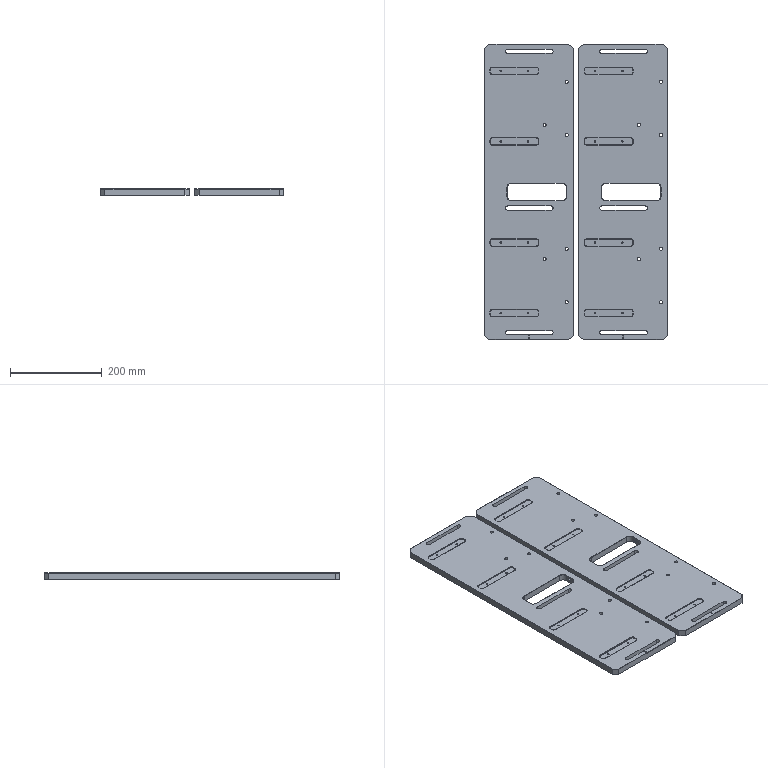NC program | NX | posted by the shop | part box 401 x 645 x 14 mm
Lines 4204 to 5636 of 5636:
N5 T02 M06
(D6 chamfer mill  D=6. R=0. H=02 ce=0.00 di=0.00)
G00 G90 G54 X-240.5 Y-185.9 M03 S3000
G43 H02 Z34.
M08
G98 G81 X-240.5 Y-185.9 Z11. R15. F200.
X-146.5 Y-137.4
X-124.5 Y-185.9
Y20.1
X-146.5 Y68.6
X-240.5 Y20.1
X124.5
X146.5 Y68.6
X240.5 Y20.1
X146.5 Y-137.4
X124.5 Y-185.9
X240.5
G80
G00 Z34.
G00 G90 X-310.789 Y102.451 M03 S6000
Z34.
Z16.934
G01 Z12.501 F1200.
X-310.731 Y102.283
X-310.7 Y102.
Y54.5
G03 X-307.5 Y51.3 I3.2 J0.0
X-304.3 Y54.5 I0.0 J3.2
G01 Y149.5
G03 X-307.5 Y152.7 I-3.2 J0.0
X-310.7 Y149.5 I0.0 J-3.2
G01 Y104.
X-310.731 Y103.717
X-310.789 Y103.549
Z16.934
G00 Z34.
X-37.372 Y102.25
Z16.099
G01 Z12.501
G03 X-37.672 Y102.33 I-.3 J-.52
X-38.192 Y102.03 I0.0 J-.6
G01 X-38.2 Y102.
Y54.5
G03 X-35. Y51.3 I3.2 J0.0
X-31.8 Y54.5 I0.0 J3.2
G01 Y149.5
G03 X-35. Y152.7 I-3.2 J0.0
X-38.2 Y149.5 I0.0 J-3.2
G01 Y102.
X-38.192 Y101.97
G03 X-37.672 Y101.67 I.52 J.3
X-37.372 Y101.75 I0.0 J.6
G01 Z16.099
G00 Z34.
X305.128 Y102.25
Z16.099
G01 Z12.501
G03 X304.828 Y102.33 I-.3 J-.52
X304.308 Y102.03 I0.0 J-.6
G01 X304.3 Y102.
Y54.5
G03 X307.5 Y51.3 I3.2 J0.0
X310.7 Y54.5 I0.0 J3.2
G01 Y149.5
G03 X307.5 Y152.7 I-3.2 J0.0
X304.3 Y149.5 I0.0 J-3.2
G01 Y102.
X304.308 Y101.97
G03 X304.828 Y101.67 I.52 J.3
X305.128 Y101.75 I0.0 J.6
G01 Z16.099
G00 Z34.
X-310.789 Y-103.549
Z16.934
G01 Z12.501
X-310.731 Y-103.717
X-310.7 Y-104.
Y-151.5
G03 X-307.5 Y-154.7 I3.2 J0.0
X-304.3 Y-151.5 I0.0 J3.2
G01 Y-56.5
G03 X-307.5 Y-53.3 I-3.2 J0.0
X-310.7 Y-56.5 I0.0 J-3.2
G01 Y-102.
X-310.731 Y-102.283
X-310.789 Y-102.451
Z16.934
G00 Z34.
X-37.372 Y-103.75
Z16.099
G01 Z12.501
G03 X-37.672 Y-103.67 I-.3 J-.52
X-38.192 Y-103.97 I0.0 J-.6
G01 X-38.2 Y-104.
Y-151.5
G03 X-35. Y-154.7 I3.2 J0.0
X-31.8 Y-151.5 I0.0 J3.2
G01 Y-56.5
G03 X-35. Y-53.3 I-3.2 J0.0
X-38.2 Y-56.5 I0.0 J-3.2
G01 Y-104.
X-38.192 Y-104.03
G03 X-37.672 Y-104.33 I.52 J.3
X-37.372 Y-104.25 I0.0 J.6
G01 Z16.099
G00 Z34.
X305.128 Y-103.75
Z16.099
G01 Z12.501
G03 X304.828 Y-103.67 I-.3 J-.52
X304.308 Y-103.97 I0.0 J-.6
G01 X304.3 Y-104.
Y-151.5
G03 X307.5 Y-154.7 I3.2 J0.0
X310.7 Y-151.5 I0.0 J3.2
G01 Y-56.5
G03 X307.5 Y-53.3 I-3.2 J0.0
X304.3 Y-56.5 I0.0 J-3.2
G01 Y-104.
X304.308 Y-104.03
G03 X304.828 Y-104.33 I.52 J.3
X305.128 Y-104.25 I0.0 J.6
G01 Z16.099
G00 Z34.
G00 G90 X-264.5 Y-101.5 M03 S5000
Z34.
G98 G81 X-264.5 Y-101.5 Z9.85 R15. F150.
Y-41.5
Y104.5
Y164.5
X-110.5
Y104.5
Y-41.5
Y-101.5
X110.5
Y-41.5
Y104.5
Y164.5
X264.5
Y104.5
Y-41.5
Y-101.5
G80
G00 Z34.
G00 G90 X-242. Y-186.895 M03 S6000
Z34.
Z12.9
G01 Z12.4 F600.
Y-187.2
G03 X-240.5 Y-188.7 I1.5 J0.0
X-237.7 Y-185.9 I0.0 J2.8
X-240.5 Y-183.1 I-2.8 J0.0
X-243.3 Y-185.9 I0.0 J-2.8
X-240.5 Y-188.7 I2.8 J0.0
X-239. Y-187.2 I0.0 J1.5
G01 Y-186.895
Z12.9
G00 Z34.
X-126.
Z12.9
G01 Z12.4
Y-187.2
G03 X-124.5 Y-188.7 I1.5 J0.0
X-121.7 Y-185.9 I0.0 J2.8
X-124.5 Y-183.1 I-2.8 J0.0
X-127.3 Y-185.9 I0.0 J-2.8
X-124.5 Y-188.7 I2.8 J0.0
X-123. Y-187.2 I0.0 J1.5
G01 Y-186.895
Z12.9
G00 Z34.
X-148. Y-138.395
Z12.9
G01 Z12.4
Y-138.7
G03 X-146.5 Y-140.2 I1.5 J0.0
X-143.7 Y-137.4 I0.0 J2.8
X-146.5 Y-134.6 I-2.8 J0.0
X-149.3 Y-137.4 I0.0 J-2.8
X-146.5 Y-140.2 I2.8 J0.0
X-145. Y-138.7 I0.0 J1.5
G01 Y-138.395
Z12.9
G00 Z34.
X-242. Y19.105
Z12.9
G01 Z12.4
Y18.8
G03 X-240.5 Y17.3 I1.5 J0.0
X-237.7 Y20.1 I0.0 J2.8
X-240.5 Y22.9 I-2.8 J0.0
X-243.3 Y20.1 I0.0 J-2.8
X-240.5 Y17.3 I2.8 J0.0
X-239. Y18.8 I0.0 J1.5
G01 Y19.105
Z12.9
G00 Z34.
X-148. Y67.605
Z12.9
G01 Z12.4
Y67.3
G03 X-146.5 Y65.8 I1.5 J0.0
X-143.7 Y68.6 I0.0 J2.8
X-146.5 Y71.4 I-2.8 J0.0
X-149.3 Y68.6 I0.0 J-2.8
X-146.5 Y65.8 I2.8 J0.0
X-145. Y67.3 I0.0 J1.5
G01 Y67.605
Z12.9
G00 Z34.
X-126. Y19.105
Z12.9
G01 Z12.4
Y18.8
G03 X-124.5 Y17.3 I1.5 J0.0
X-121.7 Y20.1 I0.0 J2.8
X-124.5 Y22.9 I-2.8 J0.0
X-127.3 Y20.1 I0.0 J-2.8
X-124.5 Y17.3 I2.8 J0.0
X-123. Y18.8 I0.0 J1.5
G01 Y19.105
Z12.9
G00 Z34.
X123.
Z12.9
G01 Z12.4
Y18.8
G03 X124.5 Y17.3 I1.5 J0.0
X127.3 Y20.1 I0.0 J2.8
X124.5 Y22.9 I-2.8 J0.0
X121.7 Y20.1 I0.0 J-2.8
X124.5 Y17.3 I2.8 J0.0
X126. Y18.8 I0.0 J1.5
G01 Y19.105
Z12.9
G00 Z34.
X145. Y67.605
Z12.9
G01 Z12.4
Y67.3
G03 X146.5 Y65.8 I1.5 J0.0
X149.3 Y68.6 I0.0 J2.8
X146.5 Y71.4 I-2.8 J0.0
X143.7 Y68.6 I0.0 J-2.8
X146.5 Y65.8 I2.8 J0.0
X148. Y67.3 I0.0 J1.5
G01 Y67.605
Z12.9
G00 Z34.
X239. Y19.105
Z12.9
G01 Z12.4
Y18.8
G03 X240.5 Y17.3 I1.5 J0.0
X243.3 Y20.1 I0.0 J2.8
X240.5 Y22.9 I-2.8 J0.0
X237.7 Y20.1 I0.0 J-2.8
X240.5 Y17.3 I2.8 J0.0
X242. Y18.8 I0.0 J1.5
G01 Y19.105
Z12.9
G00 Z34.
X145. Y-138.395
Z12.9
G01 Z12.4
Y-138.7
G03 X146.5 Y-140.2 I1.5 J0.0
X149.3 Y-137.4 I0.0 J2.8
X146.5 Y-134.6 I-2.8 J0.0
X143.7 Y-137.4 I0.0 J-2.8
X146.5 Y-140.2 I2.8 J0.0
X148. Y-138.7 I0.0 J1.5
G01 Y-138.395
Z12.9
G00 Z34.
X123. Y-186.895
Z12.9
G01 Z12.4
Y-187.2
G03 X124.5 Y-188.7 I1.5 J0.0
X127.3 Y-185.9 I0.0 J2.8
X124.5 Y-183.1 I-2.8 J0.0
X121.7 Y-185.9 I0.0 J-2.8
X124.5 Y-188.7 I2.8 J0.0
X126. Y-187.2 I0.0 J1.5
G01 Y-186.895
Z12.9
G00 Z34.
X239.
Z12.9
G01 Z12.4
Y-187.2
G03 X240.5 Y-188.7 I1.5 J0.0
X243.3 Y-185.9 I0.0 J2.8
X240.5 Y-183.1 I-2.8 J0.0
X237.7 Y-185.9 I0.0 J-2.8
X240.5 Y-188.7 I2.8 J0.0
X242. Y-187.2 I0.0 J1.5
G01 Y-186.895
Z12.9
G00 Z34.
G00 G90 X-313.126 Y4.753 M03 S6500
Z34.
Z16.501
G01 Z12.501 F1500.
X-313.354 Y4.939
X-323.061 Y14.646
X-323.247 Y14.874
Z16.501
G00 X-323.471 Y15.414
G01 Z12.501
X-323.5 Y15.707
Y102.
X-323.475 Y102.272
Z16.501
G00 Y103.728
G01 Z12.501
X-323.5 Y104.
Y190.293
X-323.471 Y190.586
Z16.501
G00 X-323.247 Y191.126
G01 Z12.501
X-323.061 Y191.354
X-313.354 Y201.061
X-313.126 Y201.247
Z16.501
G00 X-312.586 Y201.471
G01 Z12.501
X-312.293 Y201.5
X312.293
X312.586 Y201.471
Z16.501
G00 X313.126 Y201.247
G01 Z12.501
X313.354 Y201.061
X323.06 Y191.354
X323.247 Y191.126
Z16.501
G00 X323.471 Y190.586
G01 Z12.501
X323.5 Y190.293
Y15.707
X323.471 Y15.414
Z16.501
G00 X323.247 Y14.874
G01 Z12.501
X323.061 Y14.646
X313.354 Y4.939
X313.126 Y4.753
Z16.501
G00 X312.586 Y4.529
G01 Z12.501
X312.293 Y4.5
X0.0
X-312.293
X-312.586 Y4.529
Z16.501
G00 Z24.
X-304.727 Y101.614
Z13.672
G01 Z12.501
G03 X-304.527 Y101.9 I-1.532 J1.286
G01 X-304.497 Y101.946
X-304.5 Y102.
Y149.5
G03 X-307.5 Y152.5 I-3. J0.0
X-310.5 Y149.5 I0.0 J-3.
G01 Y104.
X-310.525 Y103.728
X-310.599 Y103.465
X-310.719 Y103.219
X-310.882 Y103.
X-310.719 Y102.781
X-310.599 Y102.535
X-310.525 Y102.272
X-310.5 Y102.
Y54.5
G03 X-307.5 Y51.5 I3. J0.0
X-304.5 Y54.5 I0.0 J3.
G01 Y102.
X-304.497 Y102.054
X-304.527 Y102.1
G03 X-304.727 Y102.386 I-1.732 J-1.
G01 Z13.672
G00 Z24.
X-270.873 Y134.886
Z13.672
G01 Z12.501
G03 X-271.073 Y134.6 I1.532 J-1.286
G01 X-271.103 Y134.554
X-271.1 Y134.5
Y86.5
G03 X-267.1 Y82.5 I4. J0.0
G01 X-261.9
G03 X-257.9 Y86.5 I0.0 J4.
G01 Y182.5
G03 X-261.9 Y186.5 I-4. J0.0
G01 X-267.1
G03 X-271.1 Y182.5 I0.0 J-4.
G01 Y134.5
X-271.103 Y134.446
X-271.073 Y134.4
G03 X-270.873 Y134.114 I1.732 J1.
G01 Z13.672
G00 Z24.
X-240.904 Y18.392
Z13.759
G01 Z12.501
G03 X-240.602 Y18.218 I1.147 J1.638
G01 X-240.554 Y18.192
X-240.5 Y18.2
G03 X-238.6 Y20.1 I0.0 J1.9
X-240.5 Y22. I-1.9 J0.0
X-242.4 Y20.1 I0.0 J-1.9
X-240.83 Y18.229 I1.9 J0.0
G01 X-240.5 Y18.2
X-240.446 Y18.192
X-240.398 Y18.218
G03 X-240.096 Y18.392 I-.845 J1.813
G01 Z13.759
G00 Z24.
X-124.904
Z13.759
G01 Z12.501
G03 X-124.602 Y18.218 I1.147 J1.638
G01 X-124.554 Y18.192
X-124.5 Y18.2
G03 X-122.6 Y20.1 I0.0 J1.9
X-124.5 Y22. I-1.9 J0.0
X-126.4 Y20.1 I0.0 J-1.9
X-124.83 Y18.229 I1.9 J0.0
G01 X-124.5 Y18.2
X-124.446 Y18.192
X-124.398 Y18.218
G03 X-124.096 Y18.392 I-.845 J1.813
G01 Z13.759
G00 Z24.
X-146.904 Y66.892
Z13.759
G01 Z12.501
G03 X-146.602 Y66.718 I1.147 J1.638
G01 X-146.554 Y66.692
X-146.5 Y66.7
G03 X-144.6 Y68.6 I0.0 J1.9
X-146.5 Y70.5 I-1.9 J0.0
X-148.4 Y68.6 I0.0 J-1.9
X-146.83 Y66.729 I1.9 J0.0
G01 X-146.5 Y66.7
X-146.446 Y66.692
X-146.398 Y66.718
G03 X-146.096 Y66.892 I-.845 J1.813
G01 Z13.759
G00 Z24.
X-116.873 Y134.886
Z13.672
G01 Z12.501
G03 X-117.073 Y134.6 I1.532 J-1.286
G01 X-117.103 Y134.554
X-117.1 Y134.5
Y86.5
G03 X-113.1 Y82.5 I4. J0.0
G01 X-107.9
G03 X-103.9 Y86.5 I0.0 J4.
G01 Y182.5
G03 X-107.9 Y186.5 I-4. J0.0
G01 X-113.1
G03 X-117.1 Y182.5 I0.0 J-4.
G01 Y134.5
X-117.103 Y134.446
X-117.073 Y134.4
G03 X-116.873 Y134.114 I1.732 J1.
G01 Z13.672
G00 Z24.
X-37.773 Y102.386
Z13.672
G01 Z12.501
G03 X-37.973 Y102.1 I1.532 J-1.286
G01 X-38.003 Y102.054
X-38. Y102.
Y54.5
G03 X-35. Y51.5 I3. J0.0
X-32. Y54.5 I0.0 J3.
G01 Y149.5
G03 X-35. Y152.5 I-3. J0.0
X-38. Y149.5 I0.0 J-3.
G01 Y102.
X-38.003 Y101.946
X-37.973 Y101.9
G03 X-37.773 Y101.614 I1.732 J1.
G01 Z13.672
G00 Z24.
X-17.773 Y85.886
Z13.672
G01 Z12.501
G03 X-17.973 Y85.6 I1.532 J-1.286
G01 X-18.003 Y85.554
X-18. Y85.5
Y30.5
G03 X-9. Y21.5 I9. J0.0
G01 X9.
G03 X18. Y30.5 I0.0 J9.
G01 Y140.5
G03 X9. Y149.5 I-9. J0.0
G01 X-9.
G03 X-18. Y140.5 I0.0 J-9.
G01 Y85.5
X-18.003 Y85.446
X-17.973 Y85.4
G03 X-17.773 Y85.114 I1.732 J1.
G01 Z13.672
G00 Z24.
X104.127 Y134.886
Z13.672
G01 Z12.501
G03 X103.927 Y134.6 I1.532 J-1.286
G01 X103.897 Y134.554
X103.9 Y134.5
Y86.5
G03 X107.9 Y82.5 I4. J0.0
G01 X113.1
G03 X117.1 Y86.5 I0.0 J4.
G01 Y182.5
G03 X113.1 Y186.5 I-4. J0.0
G01 X107.9
G03 X103.9 Y182.5 I0.0 J-4.
G01 Y134.5
X103.897 Y134.446
X103.927 Y134.4
G03 X104.127 Y134.114 I1.732 J1.
G01 Z13.672
G00 Z24.
X146.096 Y66.892
Z13.759
G01 Z12.501
G03 X146.398 Y66.718 I1.147 J1.638
G01 X146.446 Y66.692
X146.5 Y66.7
G03 X148.4 Y68.6 I0.0 J1.9
X146.5 Y70.5 I-1.9 J0.0
X144.6 Y68.6 I0.0 J-1.9
X146.17 Y66.729 I1.9 J0.0
G01 X146.5 Y66.7
X146.554 Y66.692
X146.602 Y66.718
G03 X146.904 Y66.892 I-.845 J1.813
G01 Z13.759
G00 Z24.
X124.096 Y18.392
Z13.759
G01 Z12.501
G03 X124.398 Y18.218 I1.147 J1.638
G01 X124.446 Y18.192
X124.5 Y18.2
G03 X126.4 Y20.1 I0.0 J1.9
X124.5 Y22. I-1.9 J0.0
X122.6 Y20.1 I0.0 J-1.9
X124.17 Y18.229 I1.9 J0.0
G01 X124.5 Y18.2
X124.554 Y18.192
X124.602 Y18.218
G03 X124.904 Y18.392 I-.845 J1.813
G01 Z13.759
G00 Z24.
X240.096
Z13.759
G01 Z12.501
G03 X240.398 Y18.218 I1.147 J1.638
G01 X240.446 Y18.192
X240.5 Y18.2
G03 X242.4 Y20.1 I0.0 J1.9
X240.5 Y22. I-1.9 J0.0
X238.6 Y20.1 I0.0 J-1.9
X240.17 Y18.229 I1.9 J0.0
G01 X240.5 Y18.2
X240.554 Y18.192
X240.602 Y18.218
G03 X240.904 Y18.392 I-.845 J1.813
G01 Z13.759
G00 Z24.
X304.727 Y102.386
Z13.672
G01 Z12.501
G03 X304.527 Y102.1 I1.532 J-1.286
G01 X304.497 Y102.054
X304.5 Y102.
Y54.5
G03 X307.5 Y51.5 I3. J0.0
X310.5 Y54.5 I0.0 J3.
G01 Y149.5
G03 X307.5 Y152.5 I-3. J0.0
X304.5 Y149.5 I0.0 J-3.
G01 Y102.
X304.497 Y101.946
X304.527 Y101.9
G03 X304.727 Y101.614 I1.732 J1.
G01 Z13.672
G00 Z24.
X270.873 Y134.114
Z13.672
G01 Z12.501
G03 X271.073 Y134.4 I-1.532 J1.286
G01 X271.103 Y134.446
X271.1 Y134.5
Y182.5
G03 X267.1 Y186.5 I-4. J0.0
G01 X261.9
G03 X257.9 Y182.5 I0.0 J-4.
G01 Y86.5
G03 X261.9 Y82.5 I4. J0.0
G01 X267.1
G03 X271.1 Y86.5 I0.0 J4.
G01 Y134.5
X271.103 Y134.554
X271.073 Y134.6
G03 X270.873 Y134.886 I-1.732 J-1.
G01 Z13.672
G00 Z24.
X313.126 Y-4.753
Z16.501
G01 Z12.501
X313.354 Y-4.939
X323.06 Y-14.646
X323.247 Y-14.874
Z16.501
G00 X323.471 Y-15.414
G01 Z12.501
X323.5 Y-15.707
Y-190.293
X323.471 Y-190.586
Z16.501
G00 X323.247 Y-191.126
G01 Z12.501
X323.061 Y-191.354
X313.354 Y-201.061
X313.126 Y-201.247
Z16.501
G00 X312.586 Y-201.471
G01 Z12.501
X312.293 Y-201.5
X-312.293
X-312.586 Y-201.471
Z16.501
G00 X-313.126 Y-201.247
G01 Z12.501
X-313.354 Y-201.061
X-323.061 Y-191.354
X-323.247 Y-191.126
Z16.501
G00 X-323.471 Y-190.586
G01 Z12.501
X-323.5 Y-190.293
Y-104.
X-323.475 Y-103.728
Z16.501
G00 Y-102.272
G01 Z12.501
X-323.5 Y-102.
Y-15.707
X-323.471 Y-15.414
Z16.501
G00 X-323.247 Y-14.874
G01 Z12.501
X-323.061 Y-14.646
X-313.354 Y-4.939
X-313.126 Y-4.753
Z16.501
G00 X-312.586 Y-4.529
G01 Z12.501
X-312.293 Y-4.5
X0.0
X312.293
X312.586 Y-4.529
Z16.501
G00 Z24.
X-304.727 Y-104.386
Z13.672
G01 Z12.501
G03 X-304.527 Y-104.1 I-1.532 J1.286
G01 X-304.497 Y-104.054
X-304.5 Y-104.
Y-56.5
G03 X-307.5 Y-53.5 I-3. J0.0
X-310.5 Y-56.5 I0.0 J-3.
G01 Y-102.
X-310.525 Y-102.272
X-310.599 Y-102.535
X-310.719 Y-102.781
X-310.882 Y-103.
X-310.719 Y-103.219
X-310.599 Y-103.465
X-310.525 Y-103.728
X-310.5 Y-104.
Y-151.5
G03 X-307.5 Y-154.5 I3. J0.0
X-304.5 Y-151.5 I0.0 J3.
G01 Y-104.
X-304.497 Y-103.946
X-304.527 Y-103.9
G03 X-304.727 Y-103.614 I-1.732 J-1.
G01 Z13.672
G00 Z24.
X-270.873 Y-71.114
Z13.672
G01 Z12.501
G03 X-271.073 Y-71.4 I1.532 J-1.286
G01 X-271.103 Y-71.446
X-271.1 Y-71.5
Y-119.5
G03 X-267.1 Y-123.5 I4. J0.0
G01 X-261.9
G03 X-257.9 Y-119.5 I0.0 J4.
G01 Y-23.5
G03 X-261.9 Y-19.5 I-4. J0.0
G01 X-267.1
G03 X-271.1 Y-23.5 I0.0 J-4.
G01 Y-71.5
X-271.103 Y-71.554
X-271.073 Y-71.6
G03 X-270.873 Y-71.886 I1.732 J1.
G01 Z13.672
G00 Z24.
X-240.904 Y-187.608
Z13.759
G01 Z12.501
G03 X-240.602 Y-187.782 I1.147 J1.638
G01 X-240.554 Y-187.808
X-240.5 Y-187.8
G03 X-238.6 Y-185.9 I0.0 J1.9
X-240.5 Y-184. I-1.9 J0.0
X-242.4 Y-185.9 I0.0 J-1.9
X-240.83 Y-187.771 I1.9 J0.0
G01 X-240.5 Y-187.8
X-240.446 Y-187.808
X-240.398 Y-187.782
G03 X-240.096 Y-187.608 I-.845 J1.813
G01 Z13.759
G00 Z24.
X-124.904
Z13.759
G01 Z12.501
G03 X-124.602 Y-187.782 I1.147 J1.638
G01 X-124.554 Y-187.808
X-124.5 Y-187.8
G03 X-122.6 Y-185.9 I0.0 J1.9
X-124.5 Y-184. I-1.9 J0.0
X-126.4 Y-185.9 I0.0 J-1.9
X-124.83 Y-187.771 I1.9 J0.0
G01 X-124.5 Y-187.8
X-124.446 Y-187.808
X-124.398 Y-187.782
G03 X-124.096 Y-187.608 I-.845 J1.813
G01 Z13.759
G00 Z24.
X-146.904 Y-139.108
Z13.759
G01 Z12.501
G03 X-146.602 Y-139.282 I1.147 J1.638
G01 X-146.554 Y-139.308
X-146.5 Y-139.3
G03 X-144.6 Y-137.4 I0.0 J1.9
X-146.5 Y-135.5 I-1.9 J0.0
X-148.4 Y-137.4 I0.0 J-1.9
X-146.83 Y-139.271 I1.9 J0.0
G01 X-146.5 Y-139.3
X-146.446 Y-139.308
X-146.398 Y-139.282
G03 X-146.096 Y-139.108 I-.845 J1.813
G01 Z13.759
G00 Z24.
X-116.873 Y-71.114
Z13.672
G01 Z12.501
G03 X-117.073 Y-71.4 I1.532 J-1.286
G01 X-117.103 Y-71.446
X-117.1 Y-71.5
Y-119.5
G03 X-113.1 Y-123.5 I4. J0.0
G01 X-107.9
G03 X-103.9 Y-119.5 I0.0 J4.
G01 Y-23.5
G03 X-107.9 Y-19.5 I-4. J0.0
G01 X-113.1
G03 X-117.1 Y-23.5 I0.0 J-4.
G01 Y-71.5
X-117.103 Y-71.554
X-117.073 Y-71.6
G03 X-116.873 Y-71.886 I1.732 J1.
G01 Z13.672
G00 Z24.
X-37.773 Y-103.614
Z13.672
G01 Z12.501
G03 X-37.973 Y-103.9 I1.532 J-1.286
G01 X-38.003 Y-103.946
X-38. Y-104.
Y-151.5
G03 X-35. Y-154.5 I3. J0.0
X-32. Y-151.5 I0.0 J3.
G01 Y-56.5
G03 X-35. Y-53.5 I-3. J0.0
X-38. Y-56.5 I0.0 J-3.
G01 Y-104.
X-38.003 Y-104.054
X-37.973 Y-104.1
G03 X-37.773 Y-104.386 I1.732 J1.
G01 Z13.672
G00 Z24.
X-17.773 Y-120.114
Z13.672
G01 Z12.501
G03 X-17.973 Y-120.4 I1.532 J-1.286
G01 X-18.003 Y-120.446
X-18. Y-120.5
Y-175.5
G03 X-9. Y-184.5 I9. J0.0
G01 X9.
G03 X18. Y-175.5 I0.0 J9.
G01 Y-65.5
G03 X9. Y-56.5 I-9. J0.0
G01 X-9.
G03 X-18. Y-65.5 I0.0 J-9.
G01 Y-120.5
X-18.003 Y-120.554
X-17.973 Y-120.6
G03 X-17.773 Y-120.886 I1.732 J1.
G01 Z13.672
G00 Z24.
X104.127 Y-71.114
Z13.672
G01 Z12.501
G03 X103.927 Y-71.4 I1.532 J-1.286
G01 X103.897 Y-71.446
X103.9 Y-71.5
Y-119.5
G03 X107.9 Y-123.5 I4. J0.0
G01 X113.1
G03 X117.1 Y-119.5 I0.0 J4.
G01 Y-23.5
G03 X113.1 Y-19.5 I-4. J0.0
G01 X107.9
G03 X103.9 Y-23.5 I0.0 J-4.
G01 Y-71.5
X103.897 Y-71.554
X103.927 Y-71.6
G03 X104.127 Y-71.886 I1.732 J1.
G01 Z13.672
G00 Z24.
X146.096 Y-139.108
Z13.759
G01 Z12.501
G03 X146.398 Y-139.282 I1.147 J1.638
G01 X146.446 Y-139.308
X146.5 Y-139.3
G03 X148.4 Y-137.4 I0.0 J1.9
X146.5 Y-135.5 I-1.9 J0.0
X144.6 Y-137.4 I0.0 J-1.9
X146.17 Y-139.271 I1.9 J0.0
G01 X146.5 Y-139.3
X146.554 Y-139.308
X146.602 Y-139.282
G03 X146.904 Y-139.108 I-.845 J1.813
G01 Z13.759
G00 Z24.
X124.096 Y-187.608
Z13.759
G01 Z12.501
G03 X124.398 Y-187.782 I1.147 J1.638
G01 X124.446 Y-187.808
X124.5 Y-187.8
G03 X126.4 Y-185.9 I0.0 J1.9
X124.5 Y-184. I-1.9 J0.0
X122.6 Y-185.9 I0.0 J-1.9
X124.17 Y-187.771 I1.9 J0.0
G01 X124.5 Y-187.8
X124.554 Y-187.808
X124.602 Y-187.782
G03 X124.904 Y-187.608 I-.845 J1.813
G01 Z13.759
G00 Z24.
X240.096
Z13.759
G01 Z12.501
G03 X240.398 Y-187.782 I1.147 J1.638
G01 X240.446 Y-187.808
X240.5 Y-187.8
G03 X242.4 Y-185.9 I0.0 J1.9
X240.5 Y-184. I-1.9 J0.0
X238.6 Y-185.9 I0.0 J-1.9
X240.17 Y-187.771 I1.9 J0.0
G01 X240.5 Y-187.8
X240.554 Y-187.808
X240.602 Y-187.782
G03 X240.904 Y-187.608 I-.845 J1.813
G01 Z13.759
G00 Z24.
X304.727 Y-103.614
Z13.672
G01 Z12.501
G03 X304.527 Y-103.9 I1.532 J-1.286
G01 X304.497 Y-103.946
X304.5 Y-104.
Y-151.5
G03 X307.5 Y-154.5 I3. J0.0
X310.5 Y-151.5 I0.0 J3.
G01 Y-56.5
G03 X307.5 Y-53.5 I-3. J0.0
X304.5 Y-56.5 I0.0 J-3.
G01 Y-104.
X304.497 Y-104.054
X304.527 Y-104.1
G03 X304.727 Y-104.386 I1.732 J1.
G01 Z13.672
G00 Z24.
X270.873 Y-71.886
Z13.672
G01 Z12.501
G03 X271.073 Y-71.6 I-1.532 J1.286
G01 X271.103 Y-71.554
X271.1 Y-71.5
Y-23.5
G03 X267.1 Y-19.5 I-4. J0.0
G01 X261.9
G03 X257.9 Y-23.5 I0.0 J-4.
G01 Y-119.5
G03 X261.9 Y-123.5 I4. J0.0
G01 X267.1
G03 X271.1 Y-119.5 I0.0 J4.
G01 Y-71.5
X271.103 Y-71.446
X271.073 Y-71.4
G03 X270.873 Y-71.114 I-1.732 J-1.
G01 Z13.672
G00 Z24.
X264.629 Y-41.436
Z11.952
G01 Z10.501
X264.531 Y-41.4
X264.5
X264.45 Y-41.413
X264.413 Y-41.45
X264.402 Y-41.517
X264.436 Y-41.577
X264.5 Y-41.6
X264.564 Y-41.577
X264.598 Y-41.517
X264.587 Y-41.45
X264.55 Y-41.413
X264.5 Y-41.4
X264.469
X264.371 Y-41.436
Z11.952
G00 Z24.
X264.629 Y-101.436
Z11.952
G01 Z10.501
X264.531 Y-101.4
X264.5
X264.45 Y-101.413
X264.413 Y-101.45
X264.402 Y-101.517
X264.436 Y-101.577
X264.5 Y-101.6
X264.564 Y-101.577
X264.598 Y-101.517
X264.587 Y-101.45
X264.55 Y-101.413
X264.5 Y-101.4
X264.469
X264.371 Y-101.436
Z11.952
G00 Z24.
X110.629 Y-41.436
Z11.952
G01 Z10.501
X110.531 Y-41.4
X110.5
X110.45 Y-41.413
X110.413 Y-41.45
X110.402 Y-41.517
X110.436 Y-41.577
X110.5 Y-41.6
X110.564 Y-41.577
X110.598 Y-41.517
X110.587 Y-41.45
X110.55 Y-41.413
X110.5 Y-41.4
X110.469
X110.371 Y-41.436
Z11.952
G00 Z24.
X110.629 Y-101.436
Z11.952
G01 Z10.501
X110.531 Y-101.4
X110.5
X110.45 Y-101.413
X110.413 Y-101.45
X110.402 Y-101.517
X110.436 Y-101.577
X110.5 Y-101.6
X110.564 Y-101.577
X110.598 Y-101.517
X110.587 Y-101.45
X110.55 Y-101.413
X110.5 Y-101.4
X110.469
X110.371 Y-101.436
Z11.952
G00 Z24.
X-110.371 Y-41.436
Z11.952
G01 Z10.501
X-110.469 Y-41.4
X-110.5
X-110.55 Y-41.413
X-110.587 Y-41.45
X-110.598 Y-41.517
X-110.564 Y-41.577
X-110.5 Y-41.6
X-110.436 Y-41.577
X-110.402 Y-41.517
X-110.413 Y-41.45
X-110.45 Y-41.413
X-110.5 Y-41.4
X-110.531
X-110.629 Y-41.436
Z11.952
G00 Z24.
X-110.371 Y-101.436
Z11.952
G01 Z10.501
X-110.469 Y-101.4
X-110.5
X-110.55 Y-101.413
X-110.587 Y-101.45
X-110.598 Y-101.517
X-110.564 Y-101.577
X-110.5 Y-101.6
X-110.436 Y-101.577
X-110.402 Y-101.517
X-110.413 Y-101.45
X-110.45 Y-101.413
X-110.5 Y-101.4
X-110.531
X-110.629 Y-101.436
Z11.952
G00 Z24.
X-264.371 Y-41.436
Z11.952
G01 Z10.501
X-264.469 Y-41.4
X-264.5
X-264.55 Y-41.413
X-264.587 Y-41.45
X-264.598 Y-41.517
X-264.564 Y-41.577
X-264.5 Y-41.6
X-264.436 Y-41.577
X-264.402 Y-41.517
X-264.413 Y-41.45
X-264.45 Y-41.413
X-264.5 Y-41.4
X-264.531
X-264.629 Y-41.436
Z11.952
G00 Z24.
X-264.371 Y-101.436
Z11.952
G01 Z10.501
X-264.469 Y-101.4
X-264.5
X-264.55 Y-101.413
X-264.587 Y-101.45
X-264.598 Y-101.517
X-264.564 Y-101.577
X-264.5 Y-101.6
X-264.436 Y-101.577
X-264.402 Y-101.517
X-264.413 Y-101.45
X-264.45 Y-101.413
X-264.5 Y-101.4
X-264.531
X-264.629 Y-101.436
Z11.952
G00 Z24.
X-264.371 Y164.564
Z11.952
G01 Z10.501
X-264.469 Y164.6
X-264.5
X-264.55 Y164.587
X-264.587 Y164.55
X-264.598 Y164.483
X-264.564 Y164.423
X-264.5 Y164.4
X-264.436 Y164.423
X-264.402 Y164.483
X-264.413 Y164.55
X-264.45 Y164.587
X-264.5 Y164.6
X-264.531
X-264.629 Y164.564
Z11.952
G00 Z24.
X-264.371 Y104.564
Z11.952
G01 Z10.501
X-264.469 Y104.6
X-264.5
X-264.55 Y104.587
X-264.587 Y104.55
X-264.598 Y104.483
X-264.564 Y104.423
X-264.5 Y104.4
X-264.436 Y104.423
X-264.402 Y104.483
X-264.413 Y104.55
X-264.45 Y104.587
X-264.5 Y104.6
X-264.531
X-264.629 Y104.564
Z11.952
G00 Z24.
X-110.371 Y164.564
Z11.952
G01 Z10.501
X-110.469 Y164.6
X-110.5
X-110.55 Y164.587
X-110.587 Y164.55
X-110.598 Y164.483
X-110.564 Y164.423
X-110.5 Y164.4
X-110.436 Y164.423
X-110.402 Y164.483
X-110.413 Y164.55
X-110.45 Y164.587
X-110.5 Y164.6
X-110.531
X-110.629 Y164.564
Z11.952
G00 Z24.
X-110.371 Y104.564
Z11.952
G01 Z10.501
X-110.469 Y104.6
X-110.5
X-110.55 Y104.587
X-110.587 Y104.55
X-110.598 Y104.483
X-110.564 Y104.423
X-110.5 Y104.4
X-110.436 Y104.423
X-110.402 Y104.483
X-110.413 Y104.55
X-110.45 Y104.587
X-110.5 Y104.6
X-110.531
X-110.629 Y104.564
Z11.952
G00 Z24.
X110.629 Y164.564
Z11.952
G01 Z10.501
X110.531 Y164.6
X110.5
X110.45 Y164.587
X110.413 Y164.55
X110.402 Y164.483
X110.436 Y164.423
X110.5 Y164.4
X110.564 Y164.423
X110.598 Y164.483
X110.587 Y164.55
X110.55 Y164.587
X110.5 Y164.6
X110.469
X110.371 Y164.564
Z11.952
G00 Z24.
X110.629 Y104.564
Z11.952
G01 Z10.501
X110.531 Y104.6
X110.5
X110.45 Y104.587
X110.413 Y104.55
X110.402 Y104.483
X110.436 Y104.423
X110.5 Y104.4
X110.564 Y104.423
X110.598 Y104.483
X110.587 Y104.55
X110.55 Y104.587
X110.5 Y104.6
X110.469
X110.371 Y104.564
Z11.952
G00 Z24.
X264.629 Y164.564
Z11.952
G01 Z10.501
X264.531 Y164.6
X264.5
X264.45 Y164.587
X264.413 Y164.55
X264.402 Y164.483
X264.436 Y164.423
X264.5 Y164.4
X264.564 Y164.423
X264.598 Y164.483
X264.587 Y164.55
X264.55 Y164.587
X264.5 Y164.6
X264.469
X264.371 Y164.564
Z11.952
G00 Z24.
X264.629 Y104.564
Z11.952
G01 Z10.501
X264.531 Y104.6
X264.5
X264.45 Y104.587
X264.413 Y104.55
X264.402 Y104.483
X264.436 Y104.423
X264.5 Y104.4
X264.564 Y104.423
X264.598 Y104.483
X264.587 Y104.55
X264.55 Y104.587
X264.5 Y104.6
X264.469
X264.371 Y104.564
Z11.952
G00 Z34.
G00 G90 X-329.5 Y103. M03 S7000
Z34.
Z15.5
G01 Z13. F300.
X-322.5
X-312.
X-305.
Z15.5
G00 Z34.
X-329.5 Y-103.
Z15.5
G01 Z13.
X-322.5
X-312.
X-305.
Z15.5
G00 Z34.
G91 G28 Z0.0
M05
M09
G91 G28 Z0.0
M01
N6 T07 M06
(D6-J  D=6. R=0. H=07 ce=0.00 di=0.00)
G00 G90 G54 X-313.517 Y204.573 M03 S6000
G43 H07 Z34.
M08
Z7.5
G01 Z7. F1000.
G41 D07
X-313.492 Y204.375
G03 X-312.5 Y203.5 I.992 J.125
G01 X312.5
G02 X314.621 Y202.621 I0.0 J-3.
G01 X324.621 Y192.621
G02 X325.5 Y190.5 I-2.121 J-2.121
G01 Y15.5
G02 X324.621 Y13.379 I-3. J0.0
G01 X314.621 Y3.379
G02 X312.5 Y2.5 I-2.121 J2.121
G01 X-312.5
G02 X-314.621 Y3.379 I0.0 J3.
G01 X-324.621 Y13.379
G02 X-325.5 Y15.5 I2.121 J2.121
G01 Y190.5
G02 X-324.621 Y192.621 I3. J0.0
G01 X-314.621 Y202.621
G02 X-312.5 Y203.5 I2.121 J-2.121
G01 X-312.
G03 X-311. Y204.5 I0.0 J1.
G01 G40 Y204.7
Z7.5
G00 Z34.
X-313.517 Y204.573
Z1.
G01 Z.5
G41 D07
X-313.492 Y204.375
G03 X-312.5 Y203.5 I.992 J.125
G01 X312.5
G02 X314.621 Y202.621 I0.0 J-3.
G01 X324.621 Y192.621
G02 X325.5 Y190.5 I-2.121 J-2.121
G01 Y15.5
G02 X324.621 Y13.379 I-3. J0.0
G01 X314.621 Y3.379
G02 X312.5 Y2.5 I-2.121 J2.121
G01 X-312.5
G02 X-314.621 Y3.379 I0.0 J3.
G01 X-324.621 Y13.379
G02 X-325.5 Y15.5 I2.121 J2.121
G01 Y190.5
G02 X-324.621 Y192.621 I3. J0.0
G01 X-314.621 Y202.621
G02 X-312.5 Y203.5 I2.121 J-2.121
G01 X-312.
G03 X-311. Y204.5 I0.0 J1.
G01 G40 Y204.7
Z1.
G00 Z34.
X313.517 Y-204.573
Z7.5
G01 Z7.
G41 D07
X313.492 Y-204.375
G03 X312.5 Y-203.5 I-.992 J-.125
G01 X-312.5
G02 X-314.621 Y-202.621 I0.0 J3.
G01 X-324.621 Y-192.621
G02 X-325.5 Y-190.5 I2.121 J2.121
G01 Y-15.5
G02 X-324.621 Y-13.379 I3. J0.0
G01 X-314.621 Y-3.379
G02 X-312.5 Y-2.5 I2.121 J-2.121
G01 X312.5
G02 X314.621 Y-3.379 I0.0 J-3.
G01 X324.621 Y-13.379
G02 X325.5 Y-15.5 I-2.121 J-2.121
G01 Y-190.5
G02 X324.621 Y-192.621 I-3. J0.0
G01 X314.621 Y-202.621
G02 X312.5 Y-203.5 I-2.121 J2.121
G01 X312.
G03 X311. Y-204.5 I0.0 J-1.
G01 G40 Y-204.7
Z7.5
G00 Z34.
X313.517 Y-204.573
Z1.
G01 Z.5
G41 D07
X313.492 Y-204.375
G03 X312.5 Y-203.5 I-.992 J-.125
G01 X-312.5
G02 X-314.621 Y-202.621 I0.0 J3.
G01 X-324.621 Y-192.621
G02 X-325.5 Y-190.5 I2.121 J2.121
G01 Y-15.5
G02 X-324.621 Y-13.379 I3. J0.0
G01 X-314.621 Y-3.379
G02 X-312.5 Y-2.5 I2.121 J-2.121
G01 X312.5
G02 X314.621 Y-3.379 I0.0 J-3.
G01 X324.621 Y-13.379
G02 X325.5 Y-15.5 I-2.121 J-2.121
G01 Y-190.5
G02 X324.621 Y-192.621 I-3. J0.0
G01 X314.621 Y-202.621
G02 X312.5 Y-203.5 I-2.121 J2.121
G01 X312.
G03 X311. Y-204.5 I0.0 J-1.
G01 G40 Y-204.7
Z1.
G00 Z34.
G00 G90 X-313.505 Y204.474 M03 S6000
Z34.
Z.7
G01 Z.2 F1000.
G41 D07
X-313.492 Y204.375
G03 X-312.5 Y203.5 I.992 J.125
G01 X312.5
G02 X314.621 Y202.621 I0.0 J-3.
G01 X324.621 Y192.621
G02 X325.5 Y190.5 I-2.121 J-2.121
G01 Y15.5
G02 X324.621 Y13.379 I-3. J0.0
G01 X314.621 Y3.379
G02 X312.5 Y2.5 I-2.121 J2.121
G01 X-312.5
G02 X-314.621 Y3.379 I0.0 J3.
G01 X-324.621 Y13.379
G02 X-325.5 Y15.5 I2.121 J2.121
G01 Y190.5
G02 X-324.621 Y192.621 I3. J0.0
G01 X-314.621 Y202.621
G02 X-312.5 Y203.5 I2.121 J-2.121
G01 X-312.
G03 X-311. Y204.5 I0.0 J1.
G01 G40 Y204.6
Z.7
G00 Z34.
X313.505 Y-204.474
Z.7
G01 Z.2
G41 D07
X313.492 Y-204.375
G03 X312.5 Y-203.5 I-.992 J-.125
G01 X-312.5
G02 X-314.621 Y-202.621 I0.0 J3.
G01 X-324.621 Y-192.621
G02 X-325.5 Y-190.5 I2.121 J2.121
G01 Y-15.5
G02 X-324.621 Y-13.379 I3. J0.0
G01 X-314.621 Y-3.379
G02 X-312.5 Y-2.5 I2.121 J-2.121
G01 X312.5
G02 X314.621 Y-3.379 I0.0 J-3.
G01 X324.621 Y-13.379
G02 X325.5 Y-15.5 I-2.121 J-2.121
G01 Y-190.5
G02 X324.621 Y-192.621 I-3. J0.0
G01 X314.621 Y-202.621
G02 X312.5 Y-203.5 I-2.121 J2.121
G01 X312.
G03 X311. Y-204.5 I0.0 J-1.
G01 G40 Y-204.6
Z.7
G00 Z34.
M05
M09
G91 G28 Z0.0
G91 G28 Y0.0
M30
%